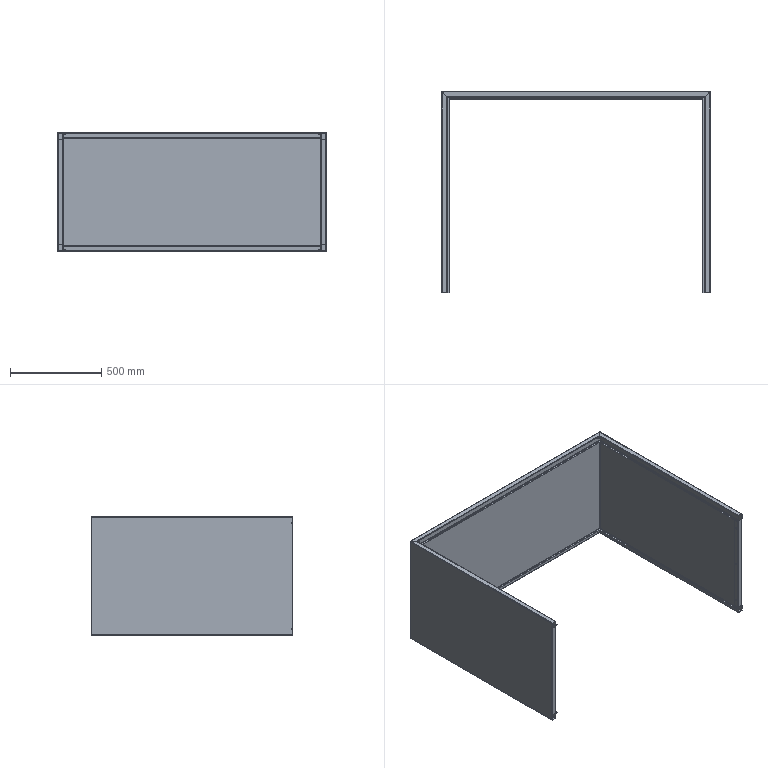Part | SolidWorks | features EdgeFlange 6, MirrorPattern 3, 3DProfileFeature 1, Cut 1, FlatPattern 1, HoleWzd 1, ICE 1, LPattern 1, SMBaseFlange 1, SheetMetal 1 | 1 solid | 268 faces | box 1470 x 1100 x 650 mm | volume 4400444 mm3 | plane 160 | cylinder 84 | spline 24 | commonest cylinder face diameters 3 x26 6 x26 4.2 x12 8.7 x12 6.2 x8